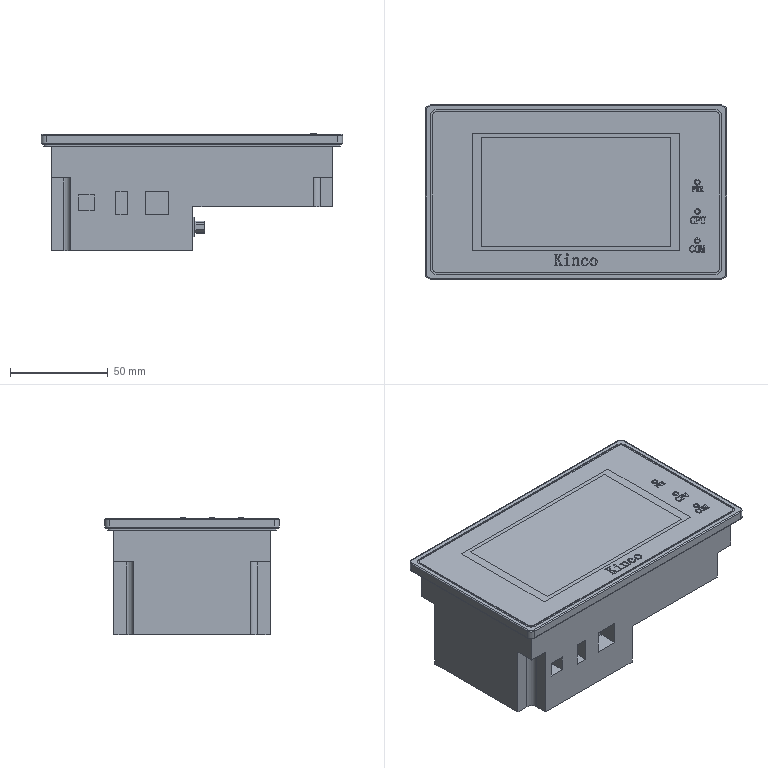Part | STEP file | Touch screen MT4200T | 1 solid | 246 faces | box 154 x 89 x 60 mm | volume 553520 mm3 | plane 142 | cylinder 66 | sphere 24 | torus 14 | commonest cylinder face diameters 0.5 x24 1 x13 4 x8 2 x5 2.5 x4 5 x4